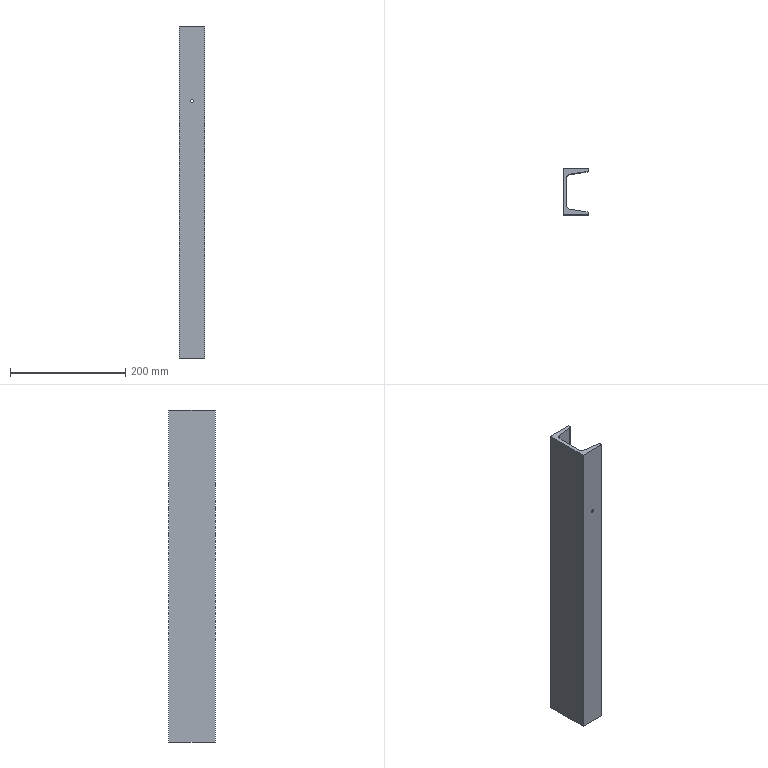Part | SolidWorks | features Extrusion 1, HoleWzd 1 | 1 solid | 18 faces | box 45 x 80 x 575 mm | volume 624060 mm3 | plane 10 | cylinder 8 | commonest cylinder face diameters 5 x4 8 x2 16 x2
STEP:
#1=CARTESIAN_POINT('',(-22.5,-72.,447.5));
#2=VERTEX_POINT('',#1);
#3=CARTESIAN_POINT('',(-22.5,-72.,442.5));
#4=VERTEX_POINT('',#3);
#5=CARTESIAN_POINT('',(-22.5,-72.,447.5));
#6=CARTESIAN_POINT('',(-27.5,-71.297,447.5));
#7=CARTESIAN_POINT('',(-27.5,-71.297,442.5));
#8=CARTESIAN_POINT('',(-22.5,-72.,442.5));
#9=(BOUNDED_CURVE()B_SPLINE_CURVE(3,(#5,#6,#7,#8),.UNSPECIFIED.,.F.,.F.)B_SPLINE_CURVE_WITH_KNOTS((4,4),(1.571,4.712),.UNSPECIFIED.)CURVE()GEOMETRIC_REPRESENTATION_ITEM()RATIONAL_B_SPLINE_CURVE((1.,0.3333,0.3333,1.))REPRESENTATION_ITEM(''));
#10=EDGE_CURVE('',#2,#4,#9,.T.);
#11=ORIENTED_EDGE('',*,*,#10,.F.);
#12=CARTESIAN_POINT('',(-22.5,-80.,447.5));
#13=VERTEX_POINT('',#12);
#14=CARTESIAN_POINT('',(-22.5,-80.,447.5));
#15=DIRECTION('',(0.,-1.,0.));
#16=VECTOR('',#15,1000.);
#17=LINE('',#14,#16);
#18=EDGE_CURVE('',#2,#13,#17,.T.);
#19=ORIENTED_EDGE('',*,*,#18,.T.);
#20=CARTESIAN_POINT('',(-22.5,-80.,442.5));
#21=VERTEX_POINT('',#20);
#22=CARTESIAN_POINT('',(-22.5,-80.,445.));
#23=DIRECTION('',(0.,-1.,0.));
#24=DIRECTION('',(0.,0.,-1.));
#25=AXIS2_PLACEMENT_3D('',#22,#23,#24);
#26=CIRCLE('',#25,2.5);
#27=EDGE_CURVE('',#13,#21,#26,.T.);
#28=ORIENTED_EDGE('',*,*,#27,.T.);
#29=CARTESIAN_POINT('',(-22.5,-80.,442.5));
#30=DIRECTION('',(0.,-1.,0.));
#31=VECTOR('',#30,1000.);
#32=LINE('',#29,#31);
#33=EDGE_CURVE('',#4,#21,#32,.T.);
#34=ORIENTED_EDGE('',*,*,#33,.F.);
#35=EDGE_LOOP('',(#11,#19,#28,#34));
#36=FACE_OUTER_BOUND('',#35,.T.);
#37=CARTESIAN_POINT('',(-22.5,-80.,445.));
#38=DIRECTION('',(0.,-1.,0.));
#39=DIRECTION('',(0.,0.,-1.));
#40=AXIS2_PLACEMENT_3D('',#37,#38,#39);
#41=CYLINDRICAL_SURFACE('',#40,2.5);
#42=ADVANCED_FACE('',(#36),#41,.F.);
#43=CARTESIAN_POINT('',(-22.5,0.,447.5));
#44=VERTEX_POINT('',#43);
#45=CARTESIAN_POINT('',(-22.5,0.,442.5));
#46=VERTEX_POINT('',#45);
#47=CARTESIAN_POINT('',(-22.5,0.,445.));
#48=DIRECTION('',(0.,-1.,0.));
#49=DIRECTION('',(0.,0.,-1.));
#50=AXIS2_PLACEMENT_3D('',#47,#48,#49);
#51=CIRCLE('',#50,2.5);
#52=EDGE_CURVE('',#44,#46,#51,.T.);
#53=ORIENTED_EDGE('',*,*,#52,.F.);
#54=CARTESIAN_POINT('',(-22.5,-8.,447.5));
#55=VERTEX_POINT('',#54);
#56=CARTESIAN_POINT('',(-22.5,-80.,447.5));
#57=DIRECTION('',(0.,-1.,0.));
#58=VECTOR('',#57,1000.);
#59=LINE('',#56,#58);
#60=EDGE_CURVE('',#44,#55,#59,.T.);
#61=ORIENTED_EDGE('',*,*,#60,.T.);
#62=CARTESIAN_POINT('',(-22.5,-8.,442.5));
#63=VERTEX_POINT('',#62);
#64=CARTESIAN_POINT('',(-22.5,-8.,442.5));
#65=CARTESIAN_POINT('',(-27.5,-8.703,442.5));
#66=CARTESIAN_POINT('',(-27.5,-8.703,447.5));
#67=CARTESIAN_POINT('',(-22.5,-8.,447.5));
#68=(BOUNDED_CURVE()B_SPLINE_CURVE(3,(#64,#65,#66,#67),.UNSPECIFIED.,.F.,.F.)B_SPLINE_CURVE_WITH_KNOTS((4,4),(4.712,7.854),.UNSPECIFIED.)CURVE()GEOMETRIC_REPRESENTATION_ITEM()RATIONAL_B_SPLINE_CURVE((1.,0.3333,0.3333,1.))REPRESENTATION_ITEM(''));
#69=EDGE_CURVE('',#63,#55,#68,.T.);
#70=ORIENTED_EDGE('',*,*,#69,.F.);
#71=CARTESIAN_POINT('',(-22.5,-80.,442.5));
#72=DIRECTION('',(0.,-1.,0.));
#73=VECTOR('',#72,1000.);
#74=LINE('',#71,#73);
#75=EDGE_CURVE('',#46,#63,#74,.T.);
#76=ORIENTED_EDGE('',*,*,#75,.F.);
#77=EDGE_LOOP('',(#53,#61,#70,#76));
#78=FACE_OUTER_BOUND('',#77,.T.);
#79=CARTESIAN_POINT('',(-22.5,-80.,445.));
#80=DIRECTION('',(0.,-1.,0.));
#81=DIRECTION('',(0.,0.,-1.));
#82=AXIS2_PLACEMENT_3D('',#79,#80,#81);
#83=CYLINDRICAL_SURFACE('',#82,2.5);
#84=ADVANCED_FACE('',(#78),#83,.F.);
#85=CARTESIAN_POINT('',(0.,-1.361,0.));
#86=VERTEX_POINT('',#85);
#87=CARTESIAN_POINT('',(0.,0.,0.));
#88=VERTEX_POINT('',#87);
#89=CARTESIAN_POINT('',(0.,-1.361,0.));
#90=DIRECTION('',(0.,1.,0.));
#91=VECTOR('',#90,1000.);
#92=LINE('',#89,#91);
#93=EDGE_CURVE('',#86,#88,#92,.T.);
#94=ORIENTED_EDGE('',*,*,#93,.T.);
#95=CARTESIAN_POINT('',(0.,0.,575.));
#96=VERTEX_POINT('',#95);
#97=CARTESIAN_POINT('',(0.,0.,575.));
#98=DIRECTION('',(0.,0.,-1.));
#99=VECTOR('',#98,1000.);
#100=LINE('',#97,#99);
#101=EDGE_CURVE('',#96,#88,#100,.T.);
#102=ORIENTED_EDGE('',*,*,#101,.F.);
#103=CARTESIAN_POINT('',(0.,-1.361,575.));
#104=VERTEX_POINT('',#103);
#105=CARTESIAN_POINT('',(0.,-1.361,575.));
#106=DIRECTION('',(0.,1.,0.));
#107=VECTOR('',#106,1000.);
#108=LINE('',#105,#107);
#109=EDGE_CURVE('',#104,#96,#108,.T.);
#110=ORIENTED_EDGE('',*,*,#109,.F.);
#111=CARTESIAN_POINT('',(0.,-1.361,575.));
#112=DIRECTION('',(0.,0.,-1.));
#113=VECTOR('',#112,1000.);
#114=LINE('',#111,#113);
#115=EDGE_CURVE('',#104,#86,#114,.T.);
#116=ORIENTED_EDGE('',*,*,#115,.T.);
#117=EDGE_LOOP('',(#94,#102,#110,#116));
#118=FACE_OUTER_BOUND('',#117,.T.);
#119=CARTESIAN_POINT('',(0.,-1.361,575.));
#120=DIRECTION('',(-1.,0.,0.));
#121=DIRECTION('',(0.,0.,1.));
#122=AXIS2_PLACEMENT_3D('',#119,#120,#121);
#123=PLANE('',#122);
#124=ADVANCED_FACE('',(#118),#123,.F.);
#125=CARTESIAN_POINT('',(-22.5,0.,445.));
#126=DIRECTION('',(0.,-1.,0.));
#127=DIRECTION('',(0.,0.,-1.));
#128=AXIS2_PLACEMENT_3D('',#125,#126,#127);
#129=CIRCLE('',#128,2.5);
#130=EDGE_CURVE('',#46,#44,#129,.T.);
#131=ORIENTED_EDGE('',*,*,#130,.T.);
#132=ORIENTED_EDGE('',*,*,#52,.T.);
#133=EDGE_LOOP('',(#131,#132));
#134=FACE_BOUND('',#133,.T.);
#135=CARTESIAN_POINT('',(-45.,0.,0.));
#136=VERTEX_POINT('',#135);
#137=CARTESIAN_POINT('',(0.,0.,0.));
#138=DIRECTION('',(-1.,0.,0.));
#139=VECTOR('',#138,1000.);
#140=LINE('',#137,#139);
#141=EDGE_CURVE('',#88,#136,#140,.T.);
#142=ORIENTED_EDGE('',*,*,#141,.T.);
#143=CARTESIAN_POINT('',(-45.,0.,575.));
#144=VERTEX_POINT('',#143);
#145=CARTESIAN_POINT('',(-45.,0.,575.));
#146=DIRECTION('',(0.,0.,-1.));
#147=VECTOR('',#146,1000.);
#148=LINE('',#145,#147);
#149=EDGE_CURVE('',#144,#136,#148,.T.);
#150=ORIENTED_EDGE('',*,*,#149,.F.);
#151=CARTESIAN_POINT('',(0.,0.,575.));
#152=DIRECTION('',(-1.,0.,0.));
#153=VECTOR('',#152,1000.);
#154=LINE('',#151,#153);
#155=EDGE_CURVE('',#96,#144,#154,.T.);
#156=ORIENTED_EDGE('',*,*,#155,.F.);
#157=ORIENTED_EDGE('',*,*,#101,.T.);
#158=EDGE_LOOP('',(#142,#150,#156,#157));
#159=FACE_OUTER_BOUND('',#158,.T.);
#160=CARTESIAN_POINT('',(0.,0.,575.));
#161=DIRECTION('',(0.,-1.,0.));
#162=DIRECTION('',(1.,0.,0.));
#163=AXIS2_PLACEMENT_3D('',#160,#161,#162);
#164=PLANE('',#163);
#165=ADVANCED_FACE('',(#134,#159),#164,.F.);
#166=CARTESIAN_POINT('',(-45.,-80.,0.));
#167=VERTEX_POINT('',#166);
#168=CARTESIAN_POINT('',(-45.,0.,0.));
#169=DIRECTION('',(0.,-1.,0.));
#170=VECTOR('',#169,1000.);
#171=LINE('',#168,#170);
#172=EDGE_CURVE('',#136,#167,#171,.T.);
#173=ORIENTED_EDGE('',*,*,#172,.T.);
#174=CARTESIAN_POINT('',(-45.,-80.,575.));
#175=VERTEX_POINT('',#174);
#176=CARTESIAN_POINT('',(-45.,-80.,575.));
#177=DIRECTION('',(0.,0.,-1.));
#178=VECTOR('',#177,1000.);
#179=LINE('',#176,#178);
#180=EDGE_CURVE('',#175,#167,#179,.T.);
#181=ORIENTED_EDGE('',*,*,#180,.F.);
#182=CARTESIAN_POINT('',(-45.,0.,575.));
#183=DIRECTION('',(0.,-1.,0.));
#184=VECTOR('',#183,1000.);
#185=LINE('',#182,#184);
#186=EDGE_CURVE('',#144,#175,#185,.T.);
#187=ORIENTED_EDGE('',*,*,#186,.F.);
#188=ORIENTED_EDGE('',*,*,#149,.T.);
#189=EDGE_LOOP('',(#173,#181,#187,#188));
#190=FACE_OUTER_BOUND('',#189,.T.);
#191=CARTESIAN_POINT('',(-45.,0.,575.));
#192=DIRECTION('',(1.,0.,0.));
#193=DIRECTION('',(0.,0.,-1.));
#194=AXIS2_PLACEMENT_3D('',#191,#192,#193);
#195=PLANE('',#194);
#196=ADVANCED_FACE('',(#190),#195,.F.);
#197=CARTESIAN_POINT('',(-22.5,-80.,445.));
#198=DIRECTION('',(0.,-1.,0.));
#199=DIRECTION('',(0.,0.,-1.));
#200=AXIS2_PLACEMENT_3D('',#197,#198,#199);
#201=CIRCLE('',#200,2.5);
#202=EDGE_CURVE('',#21,#13,#201,.T.);
#203=ORIENTED_EDGE('',*,*,#202,.F.);
#204=ORIENTED_EDGE('',*,*,#27,.F.);
#205=EDGE_LOOP('',(#203,#204));
#206=FACE_BOUND('',#205,.T.);
#207=CARTESIAN_POINT('',(0.,-80.,0.));
#208=VERTEX_POINT('',#207);
#209=CARTESIAN_POINT('',(-45.,-80.,0.));
#210=DIRECTION('',(1.,0.,0.));
#211=VECTOR('',#210,1000.);
#212=LINE('',#209,#211);
#213=EDGE_CURVE('',#167,#208,#212,.T.);
#214=ORIENTED_EDGE('',*,*,#213,.T.);
#215=CARTESIAN_POINT('',(0.,-80.,575.));
#216=VERTEX_POINT('',#215);
#217=CARTESIAN_POINT('',(0.,-80.,575.));
#218=DIRECTION('',(0.,0.,-1.));
#219=VECTOR('',#218,1000.);
#220=LINE('',#217,#219);
#221=EDGE_CURVE('',#216,#208,#220,.T.);
#222=ORIENTED_EDGE('',*,*,#221,.F.);
#223=CARTESIAN_POINT('',(-45.,-80.,575.));
#224=DIRECTION('',(1.,0.,0.));
#225=VECTOR('',#224,1000.);
#226=LINE('',#223,#225);
#227=EDGE_CURVE('',#175,#216,#226,.T.);
#228=ORIENTED_EDGE('',*,*,#227,.F.);
#229=ORIENTED_EDGE('',*,*,#180,.T.);
#230=EDGE_LOOP('',(#214,#222,#228,#229));
#231=FACE_OUTER_BOUND('',#230,.T.);
#232=CARTESIAN_POINT('',(-45.,-80.,575.));
#233=DIRECTION('',(0.,1.,0.));
#234=DIRECTION('',(0.,0.,1.));
#235=AXIS2_PLACEMENT_3D('',#232,#233,#234);
#236=PLANE('',#235);
#237=ADVANCED_FACE('',(#206,#231),#236,.F.);
#238=CARTESIAN_POINT('',(0.,-78.639,0.));
#239=VERTEX_POINT('',#238);
#240=CARTESIAN_POINT('',(0.,-80.,0.));
#241=DIRECTION('',(0.,1.,0.));
#242=VECTOR('',#241,1000.);
#243=LINE('',#240,#242);
#244=EDGE_CURVE('',#208,#239,#243,.T.);
#245=ORIENTED_EDGE('',*,*,#244,.T.);
#246=CARTESIAN_POINT('',(0.,-78.639,575.));
#247=VERTEX_POINT('',#246);
#248=CARTESIAN_POINT('',(0.,-78.639,575.));
#249=DIRECTION('',(0.,0.,-1.));
#250=VECTOR('',#249,1000.);
#251=LINE('',#248,#250);
#252=EDGE_CURVE('',#247,#239,#251,.T.);
#253=ORIENTED_EDGE('',*,*,#252,.F.);
#254=CARTESIAN_POINT('',(0.,-80.,575.));
#255=DIRECTION('',(0.,1.,0.));
#256=VECTOR('',#255,1000.);
#257=LINE('',#254,#256);
#258=EDGE_CURVE('',#216,#247,#257,.T.);
#259=ORIENTED_EDGE('',*,*,#258,.F.);
#260=ORIENTED_EDGE('',*,*,#221,.T.);
#261=EDGE_LOOP('',(#245,#253,#259,#260));
#262=FACE_OUTER_BOUND('',#261,.T.);
#263=CARTESIAN_POINT('',(0.,-80.,575.));
#264=DIRECTION('',(-1.,0.,0.));
#265=DIRECTION('',(0.,0.,1.));
#266=AXIS2_PLACEMENT_3D('',#263,#264,#265);
#267=PLANE('',#266);
#268=ADVANCED_FACE('',(#262),#267,.F.);
#269=CARTESIAN_POINT('',(-3.443,-74.678,0.));
#270=VERTEX_POINT('',#269);
#271=CARTESIAN_POINT('',(-4.,-78.639,0.));
#272=DIRECTION('',(0.,0.,1.));
#273=DIRECTION('',(1.,0.,0.));
#274=AXIS2_PLACEMENT_3D('',#271,#272,#273);
#275=CIRCLE('',#274,4.);
#276=EDGE_CURVE('',#239,#270,#275,.T.);
#277=ORIENTED_EDGE('',*,*,#276,.T.);
#278=CARTESIAN_POINT('',(-3.443,-74.678,575.));
#279=VERTEX_POINT('',#278);
#280=CARTESIAN_POINT('',(-3.443,-74.678,575.));
#281=DIRECTION('',(0.,0.,-1.));
#282=VECTOR('',#281,1000.);
#283=LINE('',#280,#282);
#284=EDGE_CURVE('',#279,#270,#283,.T.);
#285=ORIENTED_EDGE('',*,*,#284,.F.);
#286=CARTESIAN_POINT('',(-4.,-78.639,575.));
#287=DIRECTION('',(0.,0.,1.));
#288=DIRECTION('',(1.,0.,0.));
#289=AXIS2_PLACEMENT_3D('',#286,#287,#288);
#290=CIRCLE('',#289,4.);
#291=EDGE_CURVE('',#247,#279,#290,.T.);
#292=ORIENTED_EDGE('',*,*,#291,.F.);
#293=ORIENTED_EDGE('',*,*,#252,.T.);
#294=EDGE_LOOP('',(#277,#285,#292,#293));
#295=FACE_OUTER_BOUND('',#294,.T.);
#296=CARTESIAN_POINT('',(-4.,-78.639,575.));
#297=DIRECTION('',(0.,0.,-1.));
#298=DIRECTION('',(-1.,0.,0.));
#299=AXIS2_PLACEMENT_3D('',#296,#297,#298);
#300=CYLINDRICAL_SURFACE('',#299,4.);
#301=ADVANCED_FACE('',(#295),#300,.T.);
#302=CARTESIAN_POINT('',(-22.5,-72.,442.5));
#303=CARTESIAN_POINT('',(-17.5,-72.703,442.5));
#304=CARTESIAN_POINT('',(-17.5,-72.703,447.5));
#305=CARTESIAN_POINT('',(-22.5,-72.,447.5));
#306=(BOUNDED_CURVE()B_SPLINE_CURVE(3,(#302,#303,#304,#305),.UNSPECIFIED.,.F.,.F.)B_SPLINE_CURVE_WITH_KNOTS((4,4),(4.712,7.854),.UNSPECIFIED.)CURVE()GEOMETRIC_REPRESENTATION_ITEM()RATIONAL_B_SPLINE_CURVE((1.,0.3333,0.3333,1.))REPRESENTATION_ITEM(''));
#307=EDGE_CURVE('',#4,#2,#306,.T.);
#308=ORIENTED_EDGE('',*,*,#307,.T.);
#309=ORIENTED_EDGE('',*,*,#10,.T.);
#310=EDGE_LOOP('',(#308,#309));
#311=FACE_BOUND('',#310,.T.);
#312=CARTESIAN_POINT('',(-32.113,-70.649,0.));
#313=VERTEX_POINT('',#312);
#314=CARTESIAN_POINT('',(-3.443,-74.678,0.));
#315=DIRECTION('',(-0.9903,0.1392,0.));
#316=VECTOR('',#315,1000.);
#317=LINE('',#314,#316);
#318=EDGE_CURVE('',#270,#313,#317,.T.);
#319=ORIENTED_EDGE('',*,*,#318,.T.);
#320=CARTESIAN_POINT('',(-32.113,-70.649,575.));
#321=VERTEX_POINT('',#320);
#322=CARTESIAN_POINT('',(-32.113,-70.649,575.));
#323=DIRECTION('',(0.,0.,-1.));
#324=VECTOR('',#323,1000.);
#325=LINE('',#322,#324);
#326=EDGE_CURVE('',#321,#313,#325,.T.);
#327=ORIENTED_EDGE('',*,*,#326,.F.);
#328=CARTESIAN_POINT('',(-3.443,-74.678,575.));
#329=DIRECTION('',(-0.9903,0.1392,0.));
#330=VECTOR('',#329,1000.);
#331=LINE('',#328,#330);
#332=EDGE_CURVE('',#279,#321,#331,.T.);
#333=ORIENTED_EDGE('',*,*,#332,.F.);
#334=ORIENTED_EDGE('',*,*,#284,.T.);
#335=EDGE_LOOP('',(#319,#327,#333,#334));
#336=FACE_OUTER_BOUND('',#335,.T.);
#337=CARTESIAN_POINT('',(-3.443,-74.678,575.));
#338=DIRECTION('',(-0.1392,-0.9903,0.));
#339=DIRECTION('',(0.9903,-0.1392,0.));
#340=AXIS2_PLACEMENT_3D('',#337,#338,#339);
#341=PLANE('',#340);
#342=ADVANCED_FACE('',(#311,#336),#341,.F.);
#343=CARTESIAN_POINT('',(-39.,-62.727,0.));
#344=VERTEX_POINT('',#343);
#345=CARTESIAN_POINT('',(-31.,-62.727,0.));
#346=DIRECTION('',(0.,0.,-1.));
#347=DIRECTION('',(-1.,0.,0.));
#348=AXIS2_PLACEMENT_3D('',#345,#346,#347);
#349=CIRCLE('',#348,8.);
#350=EDGE_CURVE('',#313,#344,#349,.T.);
#351=ORIENTED_EDGE('',*,*,#350,.T.);
#352=CARTESIAN_POINT('',(-39.,-62.727,575.));
#353=VERTEX_POINT('',#352);
#354=CARTESIAN_POINT('',(-39.,-62.727,575.));
#355=DIRECTION('',(0.,0.,-1.));
#356=VECTOR('',#355,1000.);
#357=LINE('',#354,#356);
#358=EDGE_CURVE('',#353,#344,#357,.T.);
#359=ORIENTED_EDGE('',*,*,#358,.F.);
#360=CARTESIAN_POINT('',(-31.,-62.727,575.));
#361=DIRECTION('',(0.,0.,-1.));
#362=DIRECTION('',(-1.,0.,0.));
#363=AXIS2_PLACEMENT_3D('',#360,#361,#362);
#364=CIRCLE('',#363,8.);
#365=EDGE_CURVE('',#321,#353,#364,.T.);
#366=ORIENTED_EDGE('',*,*,#365,.F.);
#367=ORIENTED_EDGE('',*,*,#326,.T.);
#368=EDGE_LOOP('',(#351,#359,#366,#367));
#369=FACE_OUTER_BOUND('',#368,.T.);
#370=CARTESIAN_POINT('',(-31.,-62.727,575.));
#371=DIRECTION('',(0.,0.,-1.));
#372=DIRECTION('',(-1.,0.,0.));
#373=AXIS2_PLACEMENT_3D('',#370,#371,#372);
#374=CYLINDRICAL_SURFACE('',#373,8.);
#375=ADVANCED_FACE('',(#369),#374,.F.);
#376=CARTESIAN_POINT('',(-39.,-17.273,0.));
#377=VERTEX_POINT('',#376);
#378=CARTESIAN_POINT('',(-39.,-62.727,0.));
#379=DIRECTION('',(0.,1.,0.));
#380=VECTOR('',#379,1000.);
#381=LINE('',#378,#380);
#382=EDGE_CURVE('',#344,#377,#381,.T.);
#383=ORIENTED_EDGE('',*,*,#382,.T.);
#384=CARTESIAN_POINT('',(-39.,-17.273,575.));
#385=VERTEX_POINT('',#384);
#386=CARTESIAN_POINT('',(-39.,-17.273,575.));
#387=DIRECTION('',(0.,0.,-1.));
#388=VECTOR('',#387,1000.);
#389=LINE('',#386,#388);
#390=EDGE_CURVE('',#385,#377,#389,.T.);
#391=ORIENTED_EDGE('',*,*,#390,.F.);
#392=CARTESIAN_POINT('',(-39.,-62.727,575.));
#393=DIRECTION('',(0.,1.,0.));
#394=VECTOR('',#393,1000.);
#395=LINE('',#392,#394);
#396=EDGE_CURVE('',#353,#385,#395,.T.);
#397=ORIENTED_EDGE('',*,*,#396,.F.);
#398=ORIENTED_EDGE('',*,*,#358,.T.);
#399=EDGE_LOOP('',(#383,#391,#397,#398));
#400=FACE_OUTER_BOUND('',#399,.T.);
#401=CARTESIAN_POINT('',(-39.,-62.727,575.));
#402=DIRECTION('',(-1.,0.,0.));
#403=DIRECTION('',(0.,0.,1.));
#404=AXIS2_PLACEMENT_3D('',#401,#402,#403);
#405=PLANE('',#404);
#406=ADVANCED_FACE('',(#400),#405,.F.);
#407=CARTESIAN_POINT('',(-32.113,-9.351,0.));
#408=VERTEX_POINT('',#407);
#409=CARTESIAN_POINT('',(-31.,-17.273,0.));
#410=DIRECTION('',(0.,0.,-1.));
#411=DIRECTION('',(-1.,0.,0.));
#412=AXIS2_PLACEMENT_3D('',#409,#410,#411);
#413=CIRCLE('',#412,8.);
#414=EDGE_CURVE('',#377,#408,#413,.T.);
#415=ORIENTED_EDGE('',*,*,#414,.T.);
#416=CARTESIAN_POINT('',(-32.113,-9.351,575.));
#417=VERTEX_POINT('',#416);
#418=CARTESIAN_POINT('',(-32.113,-9.351,575.));
#419=DIRECTION('',(0.,0.,-1.));
#420=VECTOR('',#419,1000.);
#421=LINE('',#418,#420);
#422=EDGE_CURVE('',#417,#408,#421,.T.);
#423=ORIENTED_EDGE('',*,*,#422,.F.);
#424=CARTESIAN_POINT('',(-31.,-17.273,575.));
#425=DIRECTION('',(0.,0.,-1.));
#426=DIRECTION('',(-1.,0.,0.));
#427=AXIS2_PLACEMENT_3D('',#424,#425,#426);
#428=CIRCLE('',#427,8.);
#429=EDGE_CURVE('',#385,#417,#428,.T.);
#430=ORIENTED_EDGE('',*,*,#429,.F.);
#431=ORIENTED_EDGE('',*,*,#390,.T.);
#432=EDGE_LOOP('',(#415,#423,#430,#431));
#433=FACE_OUTER_BOUND('',#432,.T.);
#434=CARTESIAN_POINT('',(-31.,-17.273,575.));
#435=DIRECTION('',(0.,0.,-1.));
#436=DIRECTION('',(-1.,0.,0.));
#437=AXIS2_PLACEMENT_3D('',#434,#435,#436);
#438=CYLINDRICAL_SURFACE('',#437,8.);
#439=ADVANCED_FACE('',(#433),#438,.F.);
#440=ORIENTED_EDGE('',*,*,#69,.T.);
#441=CARTESIAN_POINT('',(-22.5,-8.,447.5));
#442=CARTESIAN_POINT('',(-17.5,-7.297,447.5));
#443=CARTESIAN_POINT('',(-17.5,-7.297,442.5));
#444=CARTESIAN_POINT('',(-22.5,-8.,442.5));
#445=(BOUNDED_CURVE()B_SPLINE_CURVE(3,(#441,#442,#443,#444),.UNSPECIFIED.,.F.,.F.)B_SPLINE_CURVE_WITH_KNOTS((4,4),(1.571,4.712),.UNSPECIFIED.)CURVE()GEOMETRIC_REPRESENTATION_ITEM()RATIONAL_B_SPLINE_CURVE((1.,0.3333,0.3333,1.))REPRESENTATION_ITEM(''));
#446=EDGE_CURVE('',#55,#63,#445,.T.);
#447=ORIENTED_EDGE('',*,*,#446,.T.);
#448=EDGE_LOOP('',(#440,#447));
#449=FACE_BOUND('',#448,.T.);
#450=CARTESIAN_POINT('',(-3.443,-5.322,0.));
#451=VERTEX_POINT('',#450);
#452=CARTESIAN_POINT('',(-32.113,-9.351,0.));
#453=DIRECTION('',(0.9903,0.1392,0.));
#454=VECTOR('',#453,1000.);
#455=LINE('',#452,#454);
#456=EDGE_CURVE('',#408,#451,#455,.T.);
#457=ORIENTED_EDGE('',*,*,#456,.T.);
#458=CARTESIAN_POINT('',(-3.443,-5.322,575.));
#459=VERTEX_POINT('',#458);
#460=CARTESIAN_POINT('',(-3.443,-5.322,575.));
#461=DIRECTION('',(0.,0.,-1.));
#462=VECTOR('',#461,1000.);
#463=LINE('',#460,#462);
#464=EDGE_CURVE('',#459,#451,#463,.T.);
#465=ORIENTED_EDGE('',*,*,#464,.F.);
#466=CARTESIAN_POINT('',(-32.113,-9.351,575.));
#467=DIRECTION('',(0.9903,0.1392,0.));
#468=VECTOR('',#467,1000.);
#469=LINE('',#466,#468);
#470=EDGE_CURVE('',#417,#459,#469,.T.);
#471=ORIENTED_EDGE('',*,*,#470,.F.);
#472=ORIENTED_EDGE('',*,*,#422,.T.);
#473=EDGE_LOOP('',(#457,#465,#471,#472));
#474=FACE_OUTER_BOUND('',#473,.T.);
#475=CARTESIAN_POINT('',(-32.113,-9.351,575.));
#476=DIRECTION('',(-0.1392,0.9903,0.));
#477=DIRECTION('',(-0.9903,-0.1392,0.));
#478=AXIS2_PLACEMENT_3D('',#475,#476,#477);
#479=PLANE('',#478);
#480=ADVANCED_FACE('',(#449,#474),#479,.F.);
#481=CARTESIAN_POINT('',(-4.,-1.361,0.));
#482=DIRECTION('',(0.,0.,1.));
#483=DIRECTION('',(1.,0.,0.));
#484=AXIS2_PLACEMENT_3D('',#481,#482,#483);
#485=CIRCLE('',#484,4.);
#486=EDGE_CURVE('',#451,#86,#485,.T.);
#487=ORIENTED_EDGE('',*,*,#486,.T.);
#488=ORIENTED_EDGE('',*,*,#115,.F.);
#489=CARTESIAN_POINT('',(-4.,-1.361,575.));
#490=DIRECTION('',(0.,0.,1.));
#491=DIRECTION('',(1.,0.,0.));
#492=AXIS2_PLACEMENT_3D('',#489,#490,#491);
#493=CIRCLE('',#492,4.);
#494=EDGE_CURVE('',#459,#104,#493,.T.);
#495=ORIENTED_EDGE('',*,*,#494,.F.);
#496=ORIENTED_EDGE('',*,*,#464,.T.);
#497=EDGE_LOOP('',(#487,#488,#495,#496));
#498=FACE_OUTER_BOUND('',#497,.T.);
#499=CARTESIAN_POINT('',(-4.,-1.361,575.));
#500=DIRECTION('',(0.,0.,-1.));
#501=DIRECTION('',(-1.,0.,0.));
#502=AXIS2_PLACEMENT_3D('',#499,#500,#501);
#503=CYLINDRICAL_SURFACE('',#502,4.);
#504=ADVANCED_FACE('',(#498),#503,.T.);
#505=ORIENTED_EDGE('',*,*,#109,.T.);
#506=ORIENTED_EDGE('',*,*,#155,.T.);
#507=ORIENTED_EDGE('',*,*,#186,.T.);
#508=ORIENTED_EDGE('',*,*,#227,.T.);
#509=ORIENTED_EDGE('',*,*,#258,.T.);
#510=ORIENTED_EDGE('',*,*,#291,.T.);
#511=ORIENTED_EDGE('',*,*,#332,.T.);
#512=ORIENTED_EDGE('',*,*,#365,.T.);
#513=ORIENTED_EDGE('',*,*,#396,.T.);
#514=ORIENTED_EDGE('',*,*,#429,.T.);
#515=ORIENTED_EDGE('',*,*,#470,.T.);
#516=ORIENTED_EDGE('',*,*,#494,.T.);
#517=EDGE_LOOP('',(#505,#506,#507,#508,#509,#510,#511,#512,#513,#514,#515,#516));
#518=FACE_OUTER_BOUND('',#517,.T.);
#519=CARTESIAN_POINT('',(-4.,-78.639,575.));
#520=DIRECTION('',(0.,0.,1.));
#521=DIRECTION('',(1.,0.,0.));
#522=AXIS2_PLACEMENT_3D('',#519,#520,#521);
#523=PLANE('',#522);
#524=ADVANCED_FACE('',(#518),#523,.T.);
#525=ORIENTED_EDGE('',*,*,#93,.F.);
#526=ORIENTED_EDGE('',*,*,#486,.F.);
#527=ORIENTED_EDGE('',*,*,#456,.F.);
#528=ORIENTED_EDGE('',*,*,#414,.F.);
#529=ORIENTED_EDGE('',*,*,#382,.F.);
#530=ORIENTED_EDGE('',*,*,#350,.F.);
#531=ORIENTED_EDGE('',*,*,#318,.F.);
#532=ORIENTED_EDGE('',*,*,#276,.F.);
#533=ORIENTED_EDGE('',*,*,#244,.F.);
#534=ORIENTED_EDGE('',*,*,#213,.F.);
#535=ORIENTED_EDGE('',*,*,#172,.F.);
#536=ORIENTED_EDGE('',*,*,#141,.F.);
#537=EDGE_LOOP('',(#525,#526,#527,#528,#529,#530,#531,#532,#533,#534,#535,#536));
#538=FACE_OUTER_BOUND('',#537,.T.);
#539=CARTESIAN_POINT('',(-4.,-78.639,0.));
#540=DIRECTION('',(0.,0.,1.));
#541=DIRECTION('',(1.,0.,0.));
#542=AXIS2_PLACEMENT_3D('',#539,#540,#541);
#543=PLANE('',#542);
#544=ADVANCED_FACE('',(#538),#543,.F.);
#545=ORIENTED_EDGE('',*,*,#60,.F.);
#546=ORIENTED_EDGE('',*,*,#130,.F.);
#547=ORIENTED_EDGE('',*,*,#75,.T.);
#548=ORIENTED_EDGE('',*,*,#446,.F.);
#549=EDGE_LOOP('',(#545,#546,#547,#548));
#550=FACE_OUTER_BOUND('',#549,.T.);
#551=CARTESIAN_POINT('',(-22.5,-80.,445.));
#552=DIRECTION('',(0.,-1.,0.));
#553=DIRECTION('',(0.,0.,-1.));
#554=AXIS2_PLACEMENT_3D('',#551,#552,#553);
#555=CYLINDRICAL_SURFACE('',#554,2.5);
#556=ADVANCED_FACE('',(#550),#555,.F.);
#557=ORIENTED_EDGE('',*,*,#18,.F.);
#558=ORIENTED_EDGE('',*,*,#307,.F.);
#559=ORIENTED_EDGE('',*,*,#33,.T.);
#560=ORIENTED_EDGE('',*,*,#202,.T.);
#561=EDGE_LOOP('',(#557,#558,#559,#560));
#562=FACE_OUTER_BOUND('',#561,.T.);
#563=CARTESIAN_POINT('',(-22.5,-80.,445.));
#564=DIRECTION('',(0.,-1.,0.));
#565=DIRECTION('',(0.,0.,-1.));
#566=AXIS2_PLACEMENT_3D('',#563,#564,#565);
#567=CYLINDRICAL_SURFACE('',#566,2.5);
#568=ADVANCED_FACE('',(#562),#567,.F.);
#569=CLOSED_SHELL('',(#42,#84,#124,#165,#196,#237,#268,#301,#342,#375,#406,#439,#480,#504,#524,#544,#556,#568));
#570=MANIFOLD_SOLID_BREP('',#569);
#571=CARTESIAN_POINT('',(0.,0.,0.));
#572=DIRECTION('',(0.,0.,1.));
#573=DIRECTION('',(1.,0.,0.));
#574=AXIS2_PLACEMENT_3D('',#571,#572,#573);
#575=(LENGTH_UNIT()NAMED_UNIT(*)SI_UNIT(.MILLI.,.METRE.));
#576=UNCERTAINTY_MEASURE_WITH_UNIT(LENGTH_MEASURE(0.00001),#575,'','');
#577=(NAMED_UNIT(*)PLANE_ANGLE_UNIT()SI_UNIT($,.RADIAN.));
#578=(NAMED_UNIT(*)SI_UNIT($,.STERADIAN.)SOLID_ANGLE_UNIT());
#579=(GEOMETRIC_REPRESENTATION_CONTEXT(3)GLOBAL_UNCERTAINTY_ASSIGNED_CONTEXT((#576))GLOBAL_UNIT_ASSIGNED_CONTEXT((#575,#577,#578))REPRESENTATION_CONTEXT('',''));
#580=ADVANCED_BREP_SHAPE_REPRESENTATION('',(#570,#574),#579);